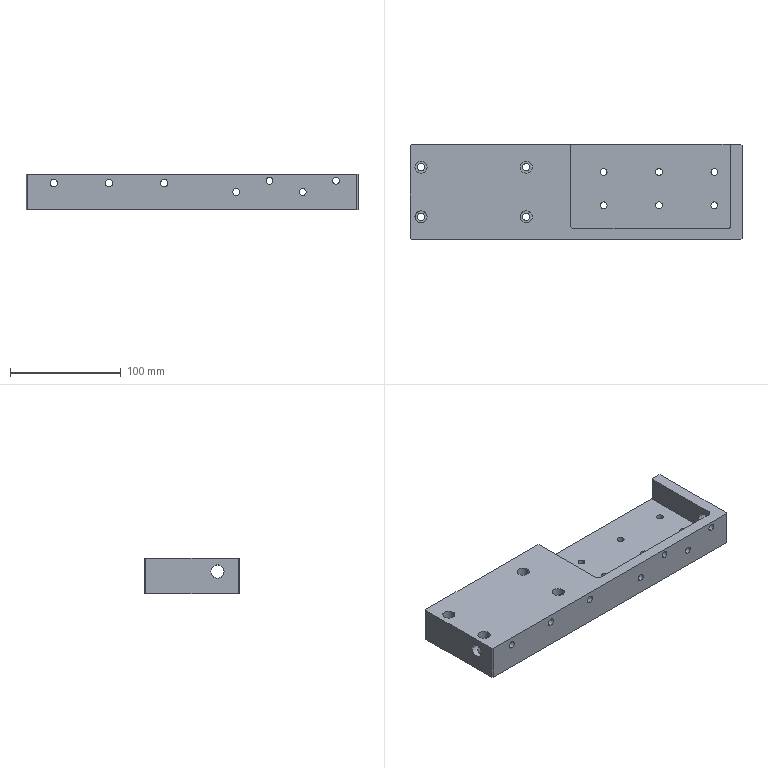Part | STEP file | X-axis connection reinforcing block | 1 solid | 88 faces | box 300 x 86 x 32 mm | volume 534000 mm3 | cylinder 63 | plane 23 | cone 2 | commonest cylinder face diameters 6.2 x20 11 x18 6.6 x14 12 x7 3.3 x2 6 x2